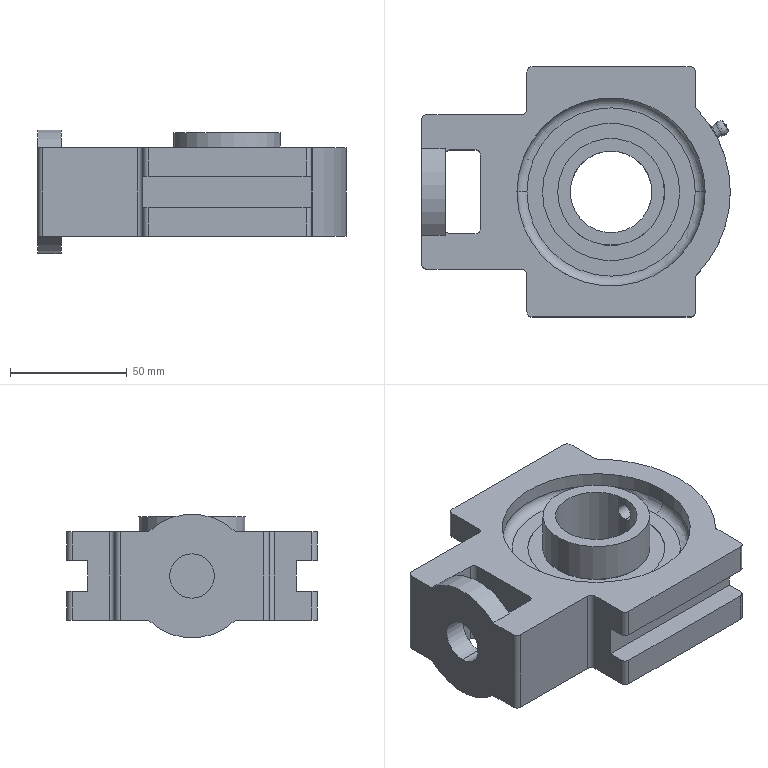Part | SolidWorks | features Revolution 6, RevCut 3, Cut 1, Extrusion 1 | 1 solid | 97 faces | box 132 x 107 x 53 mm | volume 274661 mm3 | cylinder 45 | plane 34 | torus 10 | sphere 8 | commonest cylinder face diameters 4.444 x18 45.73 x6 58.68 x6 80.5 x4 7.134 x2 19 x2